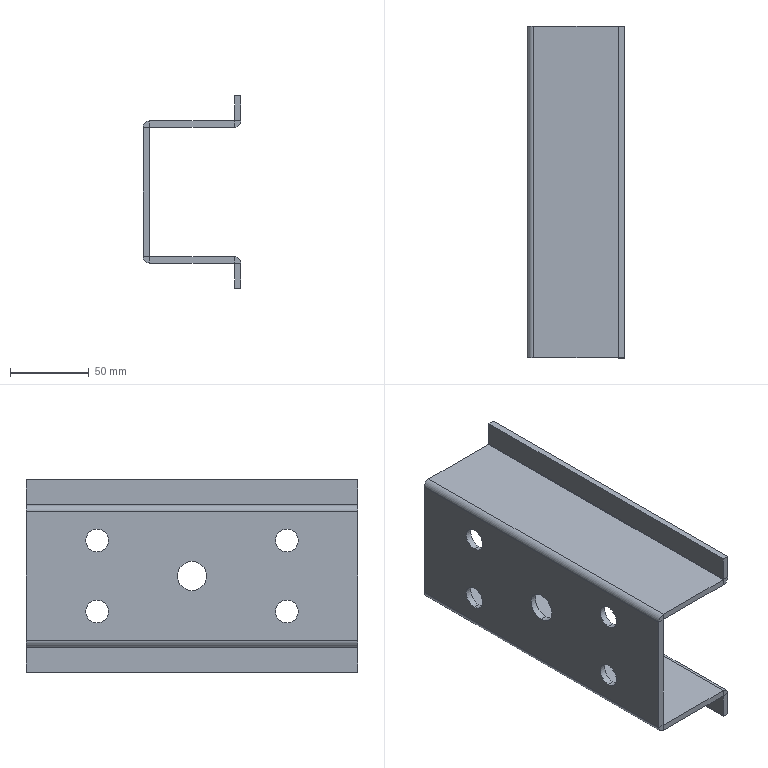Part | 1 solid | 48 faces | box 62 x 210 x 122 mm | volume 193030 mm3 | plane 30 | cylinder 18 | commonest cylinder face diameters 14.5 x8 0.4 x4 8.4 x4 18.5 x2
STEP:
#1=CARTESIAN_POINT('',(0.,0.,-9.25));
#2=VERTEX_POINT('',#1);
#3=CARTESIAN_POINT('',(0.,0.,9.25));
#4=VERTEX_POINT('',#3);
#5=CARTESIAN_POINT('',(0.,0.,0.));
#6=DIRECTION('',(-1.,0.,0.));
#7=DIRECTION('',(0.,0.,1.));
#8=AXIS2_PLACEMENT_3D('',#5,#6,#7);
#9=CIRCLE('',#8,9.25);
#10=EDGE_CURVE('',#2,#4,#9,.T.);
#11=ORIENTED_EDGE('',*,*,#10,.T.);
#12=CARTESIAN_POINT('',(4.,0.,9.25));
#13=VERTEX_POINT('',#12);
#14=CARTESIAN_POINT('',(-6.,0.,9.25));
#15=DIRECTION('',(1.,0.,0.));
#16=VECTOR('',#15,1000.);
#17=LINE('',#14,#16);
#18=EDGE_CURVE('',#4,#13,#17,.T.);
#19=ORIENTED_EDGE('',*,*,#18,.T.);
#20=CARTESIAN_POINT('',(4.,0.,-9.25));
#21=VERTEX_POINT('',#20);
#22=CARTESIAN_POINT('',(4.,0.,0.));
#23=DIRECTION('',(1.,0.,0.));
#24=DIRECTION('',(0.,0.,-1.));
#25=AXIS2_PLACEMENT_3D('',#22,#23,#24);
#26=CIRCLE('',#25,9.25);
#27=EDGE_CURVE('',#13,#21,#26,.T.);
#28=ORIENTED_EDGE('',*,*,#27,.T.);
#29=CARTESIAN_POINT('',(-6.,0.,-9.25));
#30=DIRECTION('',(1.,0.,0.));
#31=VECTOR('',#30,1000.);
#32=LINE('',#29,#31);
#33=EDGE_CURVE('',#2,#21,#32,.T.);
#34=ORIENTED_EDGE('',*,*,#33,.F.);
#35=EDGE_LOOP('',(#11,#19,#28,#34));
#36=FACE_OUTER_BOUND('',#35,.T.);
#37=CARTESIAN_POINT('',(-6.,0.,0.));
#38=DIRECTION('',(1.,0.,0.));
#39=DIRECTION('',(0.,0.,-1.));
#40=AXIS2_PLACEMENT_3D('',#37,#38,#39);
#41=CYLINDRICAL_SURFACE('',#40,9.25);
#42=ADVANCED_FACE('',(#36),#41,.F.);
#43=CARTESIAN_POINT('',(0.,-60.,-29.75));
#44=VERTEX_POINT('',#43);
#45=CARTESIAN_POINT('',(0.,-60.,-15.25));
#46=VERTEX_POINT('',#45);
#47=CARTESIAN_POINT('',(0.,-60.,-22.5));
#48=DIRECTION('',(-1.,0.,0.));
#49=DIRECTION('',(0.,0.,1.));
#50=AXIS2_PLACEMENT_3D('',#47,#48,#49);
#51=CIRCLE('',#50,7.25);
#52=EDGE_CURVE('',#44,#46,#51,.T.);
#53=ORIENTED_EDGE('',*,*,#52,.T.);
#54=CARTESIAN_POINT('',(4.,-60.,-15.25));
#55=VERTEX_POINT('',#54);
#56=CARTESIAN_POINT('',(-6.,-60.,-15.25));
#57=DIRECTION('',(1.,0.,0.));
#58=VECTOR('',#57,1000.);
#59=LINE('',#56,#58);
#60=EDGE_CURVE('',#46,#55,#59,.T.);
#61=ORIENTED_EDGE('',*,*,#60,.T.);
#62=CARTESIAN_POINT('',(4.,-60.,-29.75));
#63=VERTEX_POINT('',#62);
#64=CARTESIAN_POINT('',(4.,-60.,-22.5));
#65=DIRECTION('',(1.,0.,0.));
#66=DIRECTION('',(0.,0.,-1.));
#67=AXIS2_PLACEMENT_3D('',#64,#65,#66);
#68=CIRCLE('',#67,7.25);
#69=EDGE_CURVE('',#55,#63,#68,.T.);
#70=ORIENTED_EDGE('',*,*,#69,.T.);
#71=CARTESIAN_POINT('',(-6.,-60.,-29.75));
#72=DIRECTION('',(1.,0.,0.));
#73=VECTOR('',#72,1000.);
#74=LINE('',#71,#73);
#75=EDGE_CURVE('',#44,#63,#74,.T.);
#76=ORIENTED_EDGE('',*,*,#75,.F.);
#77=EDGE_LOOP('',(#53,#61,#70,#76));
#78=FACE_OUTER_BOUND('',#77,.T.);
#79=CARTESIAN_POINT('',(-6.,-60.,-22.5));
#80=DIRECTION('',(1.,0.,0.));
#81=DIRECTION('',(0.,0.,-1.));
#82=AXIS2_PLACEMENT_3D('',#79,#80,#81);
#83=CYLINDRICAL_SURFACE('',#82,7.25);
#84=ADVANCED_FACE('',(#78),#83,.F.);
#85=CARTESIAN_POINT('',(0.,-60.,15.25));
#86=VERTEX_POINT('',#85);
#87=CARTESIAN_POINT('',(0.,-60.,29.75));
#88=VERTEX_POINT('',#87);
#89=CARTESIAN_POINT('',(0.,-60.,22.5));
#90=DIRECTION('',(-1.,0.,0.));
#91=DIRECTION('',(0.,0.,1.));
#92=AXIS2_PLACEMENT_3D('',#89,#90,#91);
#93=CIRCLE('',#92,7.25);
#94=EDGE_CURVE('',#86,#88,#93,.T.);
#95=ORIENTED_EDGE('',*,*,#94,.T.);
#96=CARTESIAN_POINT('',(4.,-60.,29.75));
#97=VERTEX_POINT('',#96);
#98=CARTESIAN_POINT('',(-6.,-60.,29.75));
#99=DIRECTION('',(1.,0.,0.));
#100=VECTOR('',#99,1000.);
#101=LINE('',#98,#100);
#102=EDGE_CURVE('',#88,#97,#101,.T.);
#103=ORIENTED_EDGE('',*,*,#102,.T.);
#104=CARTESIAN_POINT('',(4.,-60.,15.25));
#105=VERTEX_POINT('',#104);
#106=CARTESIAN_POINT('',(4.,-60.,22.5));
#107=DIRECTION('',(1.,0.,0.));
#108=DIRECTION('',(0.,0.,-1.));
#109=AXIS2_PLACEMENT_3D('',#106,#107,#108);
#110=CIRCLE('',#109,7.25);
#111=EDGE_CURVE('',#97,#105,#110,.T.);
#112=ORIENTED_EDGE('',*,*,#111,.T.);
#113=CARTESIAN_POINT('',(-6.,-60.,15.25));
#114=DIRECTION('',(1.,0.,0.));
#115=VECTOR('',#114,1000.);
#116=LINE('',#113,#115);
#117=EDGE_CURVE('',#86,#105,#116,.T.);
#118=ORIENTED_EDGE('',*,*,#117,.F.);
#119=EDGE_LOOP('',(#95,#103,#112,#118));
#120=FACE_OUTER_BOUND('',#119,.T.);
#121=CARTESIAN_POINT('',(-6.,-60.,22.5));
#122=DIRECTION('',(1.,0.,0.));
#123=DIRECTION('',(0.,0.,-1.));
#124=AXIS2_PLACEMENT_3D('',#121,#122,#123);
#125=CYLINDRICAL_SURFACE('',#124,7.25);
#126=ADVANCED_FACE('',(#120),#125,.F.);
#127=CARTESIAN_POINT('',(0.,60.,15.25));
#128=VERTEX_POINT('',#127);
#129=CARTESIAN_POINT('',(0.,60.,29.75));
#130=VERTEX_POINT('',#129);
#131=CARTESIAN_POINT('',(0.,60.,22.5));
#132=DIRECTION('',(-1.,0.,0.));
#133=DIRECTION('',(0.,0.,1.));
#134=AXIS2_PLACEMENT_3D('',#131,#132,#133);
#135=CIRCLE('',#134,7.25);
#136=EDGE_CURVE('',#128,#130,#135,.T.);
#137=ORIENTED_EDGE('',*,*,#136,.T.);
#138=CARTESIAN_POINT('',(4.,60.,29.75));
#139=VERTEX_POINT('',#138);
#140=CARTESIAN_POINT('',(-6.,60.,29.75));
#141=DIRECTION('',(1.,0.,0.));
#142=VECTOR('',#141,1000.);
#143=LINE('',#140,#142);
#144=EDGE_CURVE('',#130,#139,#143,.T.);
#145=ORIENTED_EDGE('',*,*,#144,.T.);
#146=CARTESIAN_POINT('',(4.,60.,15.25));
#147=VERTEX_POINT('',#146);
#148=CARTESIAN_POINT('',(4.,60.,22.5));
#149=DIRECTION('',(1.,0.,0.));
#150=DIRECTION('',(0.,0.,-1.));
#151=AXIS2_PLACEMENT_3D('',#148,#149,#150);
#152=CIRCLE('',#151,7.25);
#153=EDGE_CURVE('',#139,#147,#152,.T.);
#154=ORIENTED_EDGE('',*,*,#153,.T.);
#155=CARTESIAN_POINT('',(-6.,60.,15.25));
#156=DIRECTION('',(1.,0.,0.));
#157=VECTOR('',#156,1000.);
#158=LINE('',#155,#157);
#159=EDGE_CURVE('',#128,#147,#158,.T.);
#160=ORIENTED_EDGE('',*,*,#159,.F.);
#161=EDGE_LOOP('',(#137,#145,#154,#160));
#162=FACE_OUTER_BOUND('',#161,.T.);
#163=CARTESIAN_POINT('',(-6.,60.,22.5));
#164=DIRECTION('',(1.,0.,0.));
#165=DIRECTION('',(0.,0.,-1.));
#166=AXIS2_PLACEMENT_3D('',#163,#164,#165);
#167=CYLINDRICAL_SURFACE('',#166,7.25);
#168=ADVANCED_FACE('',(#162),#167,.F.);
#169=CARTESIAN_POINT('',(0.,60.,-29.75));
#170=VERTEX_POINT('',#169);
#171=CARTESIAN_POINT('',(0.,60.,-15.25));
#172=VERTEX_POINT('',#171);
#173=CARTESIAN_POINT('',(0.,60.,-22.5));
#174=DIRECTION('',(-1.,0.,0.));
#175=DIRECTION('',(0.,0.,1.));
#176=AXIS2_PLACEMENT_3D('',#173,#174,#175);
#177=CIRCLE('',#176,7.25);
#178=EDGE_CURVE('',#170,#172,#177,.T.);
#179=ORIENTED_EDGE('',*,*,#178,.T.);
#180=CARTESIAN_POINT('',(4.,60.,-15.25));
#181=VERTEX_POINT('',#180);
#182=CARTESIAN_POINT('',(-6.,60.,-15.25));
#183=DIRECTION('',(1.,0.,0.));
#184=VECTOR('',#183,1000.);
#185=LINE('',#182,#184);
#186=EDGE_CURVE('',#172,#181,#185,.T.);
#187=ORIENTED_EDGE('',*,*,#186,.T.);
#188=CARTESIAN_POINT('',(4.,60.,-29.75));
#189=VERTEX_POINT('',#188);
#190=CARTESIAN_POINT('',(4.,60.,-22.5));
#191=DIRECTION('',(1.,0.,0.));
#192=DIRECTION('',(0.,0.,-1.));
#193=AXIS2_PLACEMENT_3D('',#190,#191,#192);
#194=CIRCLE('',#193,7.25);
#195=EDGE_CURVE('',#181,#189,#194,.T.);
#196=ORIENTED_EDGE('',*,*,#195,.T.);
#197=CARTESIAN_POINT('',(-6.,60.,-29.75));
#198=DIRECTION('',(1.,0.,0.));
#199=VECTOR('',#198,1000.);
#200=LINE('',#197,#199);
#201=EDGE_CURVE('',#170,#189,#200,.T.);
#202=ORIENTED_EDGE('',*,*,#201,.F.);
#203=EDGE_LOOP('',(#179,#187,#196,#202));
#204=FACE_OUTER_BOUND('',#203,.T.);
#205=CARTESIAN_POINT('',(-6.,60.,-22.5));
#206=DIRECTION('',(1.,0.,0.));
#207=DIRECTION('',(0.,0.,-1.));
#208=AXIS2_PLACEMENT_3D('',#205,#206,#207);
#209=CYLINDRICAL_SURFACE('',#208,7.25);
#210=ADVANCED_FACE('',(#204),#209,.F.);
#211=CARTESIAN_POINT('',(57.8,-105.,45.));
#212=VERTEX_POINT('',#211);
#213=CARTESIAN_POINT('',(4.2,-105.,45.));
#214=VERTEX_POINT('',#213);
#215=CARTESIAN_POINT('',(0.,-105.,45.));
#216=DIRECTION('',(-1.,0.,0.));
#217=VECTOR('',#216,1000.);
#218=LINE('',#215,#217);
#219=EDGE_CURVE('',#212,#214,#218,.T.);
#220=ORIENTED_EDGE('',*,*,#219,.F.);
#221=CARTESIAN_POINT('',(57.8,105.,45.));
#222=VERTEX_POINT('',#221);
#223=CARTESIAN_POINT('',(57.8,105.,45.));
#224=DIRECTION('',(0.,-1.,0.));
#225=VECTOR('',#224,1000.);
#226=LINE('',#223,#225);
#227=EDGE_CURVE('',#222,#212,#226,.T.);
#228=ORIENTED_EDGE('',*,*,#227,.F.);
#229=CARTESIAN_POINT('',(4.2,105.,45.));
#230=VERTEX_POINT('',#229);
#231=CARTESIAN_POINT('',(0.,105.,45.));
#232=DIRECTION('',(-1.,0.,0.));
#233=VECTOR('',#232,1000.);
#234=LINE('',#231,#233);
#235=EDGE_CURVE('',#222,#230,#234,.T.);
#236=ORIENTED_EDGE('',*,*,#235,.T.);
#237=CARTESIAN_POINT('',(4.2,105.,45.));
#238=DIRECTION('',(0.,-1.,0.));
#239=VECTOR('',#238,1000.);
#240=LINE('',#237,#239);
#241=EDGE_CURVE('',#230,#214,#240,.T.);
#242=ORIENTED_EDGE('',*,*,#241,.T.);
#243=EDGE_LOOP('',(#220,#228,#236,#242));
#244=FACE_OUTER_BOUND('',#243,.T.);
#245=CARTESIAN_POINT('',(0.,105.,45.));
#246=DIRECTION('',(0.,0.,1.));
#247=DIRECTION('',(1.,0.,0.));
#248=AXIS2_PLACEMENT_3D('',#245,#246,#247);
#249=PLANE('',#248);
#250=ADVANCED_FACE('',(#244),#249,.T.);
#251=CARTESIAN_POINT('',(57.8,105.,41.));
#252=VERTEX_POINT('',#251);
#253=CARTESIAN_POINT('',(57.8,-105.,41.));
#254=VERTEX_POINT('',#253);
#255=CARTESIAN_POINT('',(57.8,105.,41.));
#256=DIRECTION('',(0.,-1.,0.));
#257=VECTOR('',#256,1000.);
#258=LINE('',#255,#257);
#259=EDGE_CURVE('',#252,#254,#258,.T.);
#260=ORIENTED_EDGE('',*,*,#259,.T.);
#261=CARTESIAN_POINT('',(4.2,-105.,41.));
#262=VERTEX_POINT('',#261);
#263=CARTESIAN_POINT('',(0.,-105.,41.));
#264=DIRECTION('',(-1.,0.,0.));
#265=VECTOR('',#264,1000.);
#266=LINE('',#263,#265);
#267=EDGE_CURVE('',#254,#262,#266,.T.);
#268=ORIENTED_EDGE('',*,*,#267,.T.);
#269=CARTESIAN_POINT('',(4.2,105.,41.));
#270=VERTEX_POINT('',#269);
#271=CARTESIAN_POINT('',(4.2,105.,41.));
#272=DIRECTION('',(0.,-1.,0.));
#273=VECTOR('',#272,1000.);
#274=LINE('',#271,#273);
#275=EDGE_CURVE('',#270,#262,#274,.T.);
#276=ORIENTED_EDGE('',*,*,#275,.F.);
#277=CARTESIAN_POINT('',(0.,105.,41.));
#278=DIRECTION('',(-1.,0.,0.));
#279=VECTOR('',#278,1000.);
#280=LINE('',#277,#279);
#281=EDGE_CURVE('',#252,#270,#280,.T.);
#282=ORIENTED_EDGE('',*,*,#281,.F.);
#283=EDGE_LOOP('',(#260,#268,#276,#282));
#284=FACE_OUTER_BOUND('',#283,.T.);
#285=CARTESIAN_POINT('',(0.,105.,41.));
#286=DIRECTION('',(0.,0.,1.));
#287=DIRECTION('',(1.,0.,0.));
#288=AXIS2_PLACEMENT_3D('',#285,#286,#287);
#289=PLANE('',#288);
#290=ADVANCED_FACE('',(#284),#289,.F.);
#291=ORIENTED_EDGE('',*,*,#235,.F.);
#292=CARTESIAN_POINT('',(57.8,105.,45.));
#293=DIRECTION('',(0.,0.,-1.));
#294=VECTOR('',#293,1000.);
#295=LINE('',#292,#294);
#296=EDGE_CURVE('',#222,#252,#295,.T.);
#297=ORIENTED_EDGE('',*,*,#296,.T.);
#298=ORIENTED_EDGE('',*,*,#281,.T.);
#299=CARTESIAN_POINT('',(4.2,105.,41.));
#300=DIRECTION('',(0.,0.,1.));
#301=VECTOR('',#300,1000.);
#302=LINE('',#299,#301);
#303=EDGE_CURVE('',#270,#230,#302,.T.);
#304=ORIENTED_EDGE('',*,*,#303,.T.);
#305=EDGE_LOOP('',(#291,#297,#298,#304));
#306=FACE_OUTER_BOUND('',#305,.T.);
#307=CARTESIAN_POINT('',(4.2,105.,-40.8));
#308=DIRECTION('',(0.,1.,0.));
#309=DIRECTION('',(1.,0.,0.));
#310=AXIS2_PLACEMENT_3D('',#307,#308,#309);
#311=PLANE('',#310);
#312=ADVANCED_FACE('',(#306),#311,.T.);
#313=CARTESIAN_POINT('',(57.8,-105.,-41.));
#314=VERTEX_POINT('',#313);
#315=CARTESIAN_POINT('',(57.8,105.,-41.));
#316=VERTEX_POINT('',#315);
#317=CARTESIAN_POINT('',(57.8,-105.,-41.));
#318=DIRECTION('',(0.,1.,0.));
#319=VECTOR('',#318,1000.);
#320=LINE('',#317,#319);
#321=EDGE_CURVE('',#314,#316,#320,.T.);
#322=ORIENTED_EDGE('',*,*,#321,.T.);
#323=CARTESIAN_POINT('',(4.2,105.,-41.));
#324=VERTEX_POINT('',#323);
#325=CARTESIAN_POINT('',(0.,105.,-41.));
#326=DIRECTION('',(1.,0.,0.));
#327=VECTOR('',#326,1000.);
#328=LINE('',#325,#327);
#329=EDGE_CURVE('',#324,#316,#328,.T.);
#330=ORIENTED_EDGE('',*,*,#329,.F.);
#331=CARTESIAN_POINT('',(4.2,-105.,-41.));
#332=VERTEX_POINT('',#331);
#333=CARTESIAN_POINT('',(4.2,105.,-41.));
#334=DIRECTION('',(0.,-1.,0.));
#335=VECTOR('',#334,1000.);
#336=LINE('',#333,#335);
#337=EDGE_CURVE('',#324,#332,#336,.T.);
#338=ORIENTED_EDGE('',*,*,#337,.T.);
#339=CARTESIAN_POINT('',(0.,-105.,-41.));
#340=DIRECTION('',(1.,0.,0.));
#341=VECTOR('',#340,1000.);
#342=LINE('',#339,#341);
#343=EDGE_CURVE('',#332,#314,#342,.T.);
#344=ORIENTED_EDGE('',*,*,#343,.T.);
#345=EDGE_LOOP('',(#322,#330,#338,#344));
#346=FACE_OUTER_BOUND('',#345,.T.);
#347=CARTESIAN_POINT('',(0.,105.,-41.));
#348=DIRECTION('',(0.,0.,-1.));
#349=DIRECTION('',(-1.,0.,0.));
#350=AXIS2_PLACEMENT_3D('',#347,#348,#349);
#351=PLANE('',#350);
#352=ADVANCED_FACE('',(#346),#351,.F.);
#353=CARTESIAN_POINT('',(4.2,105.,-45.));
#354=VERTEX_POINT('',#353);
#355=CARTESIAN_POINT('',(57.8,105.,-45.));
#356=VERTEX_POINT('',#355);
#357=CARTESIAN_POINT('',(0.,105.,-45.));
#358=DIRECTION('',(1.,0.,0.));
#359=VECTOR('',#358,1000.);
#360=LINE('',#357,#359);
#361=EDGE_CURVE('',#354,#356,#360,.T.);
#362=ORIENTED_EDGE('',*,*,#361,.T.);
#363=CARTESIAN_POINT('',(57.8,-105.,-45.));
#364=VERTEX_POINT('',#363);
#365=CARTESIAN_POINT('',(57.8,-105.,-45.));
#366=DIRECTION('',(0.,1.,0.));
#367=VECTOR('',#366,1000.);
#368=LINE('',#365,#367);
#369=EDGE_CURVE('',#364,#356,#368,.T.);
#370=ORIENTED_EDGE('',*,*,#369,.F.);
#371=CARTESIAN_POINT('',(4.2,-105.,-45.));
#372=VERTEX_POINT('',#371);
#373=CARTESIAN_POINT('',(0.,-105.,-45.));
#374=DIRECTION('',(1.,0.,0.));
#375=VECTOR('',#374,1000.);
#376=LINE('',#373,#375);
#377=EDGE_CURVE('',#372,#364,#376,.T.);
#378=ORIENTED_EDGE('',*,*,#377,.F.);
#379=CARTESIAN_POINT('',(4.2,105.,-45.));
#380=DIRECTION('',(0.,-1.,0.));
#381=VECTOR('',#380,1000.);
#382=LINE('',#379,#381);
#383=EDGE_CURVE('',#354,#372,#382,.T.);
#384=ORIENTED_EDGE('',*,*,#383,.F.);
#385=EDGE_LOOP('',(#362,#370,#378,#384));
#386=FACE_OUTER_BOUND('',#385,.T.);
#387=CARTESIAN_POINT('',(0.,105.,-45.));
#388=DIRECTION('',(0.,0.,-1.));
#389=DIRECTION('',(-1.,0.,0.));
#390=AXIS2_PLACEMENT_3D('',#387,#388,#389);
#391=PLANE('',#390);
#392=ADVANCED_FACE('',(#386),#391,.T.);
#393=CARTESIAN_POINT('',(57.8,-105.,-45.));
#394=DIRECTION('',(0.,0.,1.));
#395=VECTOR('',#394,1000.);
#396=LINE('',#393,#395);
#397=EDGE_CURVE('',#364,#314,#396,.T.);
#398=ORIENTED_EDGE('',*,*,#397,.T.);
#399=ORIENTED_EDGE('',*,*,#343,.F.);
#400=CARTESIAN_POINT('',(4.2,-105.,-41.));
#401=DIRECTION('',(0.,0.,-1.));
#402=VECTOR('',#401,1000.);
#403=LINE('',#400,#402);
#404=EDGE_CURVE('',#332,#372,#403,.T.);
#405=ORIENTED_EDGE('',*,*,#404,.T.);
#406=ORIENTED_EDGE('',*,*,#377,.T.);
#407=EDGE_LOOP('',(#398,#399,#405,#406));
#408=FACE_OUTER_BOUND('',#407,.T.);
#409=CARTESIAN_POINT('',(4.2,-105.,-40.8));
#410=DIRECTION('',(0.,1.,0.));
#411=DIRECTION('',(1.,0.,0.));
#412=AXIS2_PLACEMENT_3D('',#409,#410,#411);
#413=PLANE('',#412);
#414=ADVANCED_FACE('',(#408),#413,.F.);
#415=CARTESIAN_POINT('',(0.,105.,40.8));
#416=VERTEX_POINT('',#415);
#417=CARTESIAN_POINT('',(4.,105.,40.8));
#418=VERTEX_POINT('',#417);
#419=CARTESIAN_POINT('',(0.,105.,40.8));
#420=DIRECTION('',(1.,0.,0.));
#421=VECTOR('',#420,1000.);
#422=LINE('',#419,#421);
#423=EDGE_CURVE('',#416,#418,#422,.T.);
#424=ORIENTED_EDGE('',*,*,#423,.F.);
#425=CARTESIAN_POINT('',(4.2,105.,40.8));
#426=DIRECTION('',(0.,-1.,0.));
#427=DIRECTION('',(0.,0.,1.));
#428=AXIS2_PLACEMENT_3D('',#425,#426,#427);
#429=CIRCLE('',#428,4.2);
#430=EDGE_CURVE('',#230,#416,#429,.T.);
#431=ORIENTED_EDGE('',*,*,#430,.F.);
#432=ORIENTED_EDGE('',*,*,#303,.F.);
#433=CARTESIAN_POINT('',(4.2,105.,40.8));
#434=DIRECTION('',(0.,-1.,0.));
#435=DIRECTION('',(1.,0.,0.));
#436=AXIS2_PLACEMENT_3D('',#433,#434,#435);
#437=CIRCLE('',#436,0.2);
#438=EDGE_CURVE('',#270,#418,#437,.T.);
#439=ORIENTED_EDGE('',*,*,#438,.T.);
#440=EDGE_LOOP('',(#424,#431,#432,#439));
#441=FACE_OUTER_BOUND('',#440,.T.);
#442=CARTESIAN_POINT('',(0.,105.,40.8));
#443=DIRECTION('',(0.,1.,0.));
#444=DIRECTION('',(0.,0.,1.));
#445=AXIS2_PLACEMENT_3D('',#442,#443,#444);
#446=PLANE('',#445);
#447=ADVANCED_FACE('',(#441),#446,.T.);
#448=CARTESIAN_POINT('',(0.,105.,-40.8));
#449=VERTEX_POINT('',#448);
#450=CARTESIAN_POINT('',(0.,105.,-45.));
#451=DIRECTION('',(0.,0.,-1.));
#452=VECTOR('',#451,1000.);
#453=LINE('',#450,#452);
#454=EDGE_CURVE('',#416,#449,#453,.T.);
#455=ORIENTED_EDGE('',*,*,#454,.F.);
#456=ORIENTED_EDGE('',*,*,#423,.T.);
#457=CARTESIAN_POINT('',(4.,105.,-40.8));
#458=VERTEX_POINT('',#457);
#459=CARTESIAN_POINT('',(4.,105.,-45.));
#460=DIRECTION('',(0.,0.,-1.));
#461=VECTOR('',#460,1000.);
#462=LINE('',#459,#461);
#463=EDGE_CURVE('',#418,#458,#462,.T.);
#464=ORIENTED_EDGE('',*,*,#463,.T.);
#465=CARTESIAN_POINT('',(4.,105.,-40.8));
#466=DIRECTION('',(-1.,0.,0.));
#467=VECTOR('',#466,1000.);
#468=LINE('',#465,#467);
#469=EDGE_CURVE('',#458,#449,#468,.T.);
#470=ORIENTED_EDGE('',*,*,#469,.T.);
#471=EDGE_LOOP('',(#455,#456,#464,#470));
#472=FACE_OUTER_BOUND('',#471,.T.);
#473=CARTESIAN_POINT('',(4.2,105.,41.));
#474=DIRECTION('',(0.,1.,0.));
#475=DIRECTION('',(0.,0.,1.));
#476=AXIS2_PLACEMENT_3D('',#473,#474,#475);
#477=PLANE('',#476);
#478=ADVANCED_FACE('',(#472),#477,.T.);
#479=CARTESIAN_POINT('',(4.2,-105.,45.));
#480=DIRECTION('',(0.,0.,-1.));
#481=VECTOR('',#480,1000.);
#482=LINE('',#479,#481);
#483=EDGE_CURVE('',#214,#262,#482,.T.);
#484=ORIENTED_EDGE('',*,*,#483,.F.);
#485=CARTESIAN_POINT('',(0.,-105.,40.8));
#486=VERTEX_POINT('',#485);
#487=CARTESIAN_POINT('',(4.2,-105.,40.8));
#488=DIRECTION('',(0.,-1.,0.));
#489=DIRECTION('',(0.,0.,1.));
#490=AXIS2_PLACEMENT_3D('',#487,#488,#489);
#491=CIRCLE('',#490,4.2);
#492=EDGE_CURVE('',#214,#486,#491,.T.);
#493=ORIENTED_EDGE('',*,*,#492,.T.);
#494=CARTESIAN_POINT('',(4.,-105.,40.8));
#495=VERTEX_POINT('',#494);
#496=CARTESIAN_POINT('',(4.,-105.,40.8));
#497=DIRECTION('',(-1.,0.,0.));
#498=VECTOR('',#497,1000.);
#499=LINE('',#496,#498);
#500=EDGE_CURVE('',#495,#486,#499,.T.);
#501=ORIENTED_EDGE('',*,*,#500,.F.);
#502=CARTESIAN_POINT('',(4.2,-105.,40.8));
#503=DIRECTION('',(0.,-1.,0.));
#504=DIRECTION('',(1.,0.,0.));
#505=AXIS2_PLACEMENT_3D('',#502,#503,#504);
#506=CIRCLE('',#505,0.2);
#507=EDGE_CURVE('',#262,#495,#506,.T.);
#508=ORIENTED_EDGE('',*,*,#507,.F.);
#509=EDGE_LOOP('',(#484,#493,#501,#508));
#510=FACE_OUTER_BOUND('',#509,.T.);
#511=CARTESIAN_POINT('',(4.2,-105.,45.));
#512=DIRECTION('',(0.,-1.,0.));
#513=DIRECTION('',(0.,0.,-1.));
#514=AXIS2_PLACEMENT_3D('',#511,#512,#513);
#515=PLANE('',#514);
#516=ADVANCED_FACE('',(#510),#515,.T.);
#517=CARTESIAN_POINT('',(57.8,-105.,45.));
#518=DIRECTION('',(0.,0.,-1.));
#519=VECTOR('',#518,1000.);
#520=LINE('',#517,#519);
#521=EDGE_CURVE('',#212,#254,#520,.T.);
#522=ORIENTED_EDGE('',*,*,#521,.F.);
#523=ORIENTED_EDGE('',*,*,#219,.T.);
#524=ORIENTED_EDGE('',*,*,#483,.T.);
#525=ORIENTED_EDGE('',*,*,#267,.F.);
#526=EDGE_LOOP('',(#522,#523,#524,#525));
#527=FACE_OUTER_BOUND('',#526,.T.);
#528=CARTESIAN_POINT('',(4.,-105.,40.8));
#529=DIRECTION('',(0.,-1.,0.));
#530=DIRECTION('',(0.,0.,-1.));
#531=AXIS2_PLACEMENT_3D('',#528,#529,#530);
#532=PLANE('',#531);
#533=ADVANCED_FACE('',(#527),#532,.T.);
#534=CARTESIAN_POINT('',(4.2,105.,-45.));
#535=DIRECTION('',(0.,0.,1.));
#536=VECTOR('',#535,1000.);
#537=LINE('',#534,#536);
#538=EDGE_CURVE('',#354,#324,#537,.T.);
#539=ORIENTED_EDGE('',*,*,#538,.F.);
#540=CARTESIAN_POINT('',(4.2,105.,-40.8));
#541=DIRECTION('',(0.,-1.,0.));
#542=DIRECTION('',(0.,0.,1.));
#543=AXIS2_PLACEMENT_3D('',#540,#541,#542);
#544=CIRCLE('',#543,4.2);
#545=EDGE_CURVE('',#449,#354,#544,.T.);
#546=ORIENTED_EDGE('',*,*,#545,.F.);
#547=ORIENTED_EDGE('',*,*,#469,.F.);
#548=CARTESIAN_POINT('',(4.2,105.,-40.8));
#549=DIRECTION('',(0.,-1.,0.));
#550=DIRECTION('',(1.,0.,0.));
#551=AXIS2_PLACEMENT_3D('',#548,#549,#550);
#552=CIRCLE('',#551,0.2);
#553=EDGE_CURVE('',#458,#324,#552,.T.);
#554=ORIENTED_EDGE('',*,*,#553,.T.);
#555=EDGE_LOOP('',(#539,#546,#547,#554));
#556=FACE_OUTER_BOUND('',#555,.T.);
#557=CARTESIAN_POINT('',(4.2,105.,-45.));
#558=DIRECTION('',(0.,1.,0.));
#559=DIRECTION('',(0.,0.,1.));
#560=AXIS2_PLACEMENT_3D('',#557,#558,#559);
#561=PLANE('',#560);
#562=ADVANCED_FACE('',(#556),#561,.T.);
#563=CARTESIAN_POINT('',(57.8,105.,-45.));
#564=DIRECTION('',(0.,0.,1.));
#565=VECTOR('',#564,1000.);
#566=LINE('',#563,#565);
#567=EDGE_CURVE('',#356,#316,#566,.T.);
#568=ORIENTED_EDGE('',*,*,#567,.F.);
#569=ORIENTED_EDGE('',*,*,#361,.F.);
#570=ORIENTED_EDGE('',*,*,#538,.T.);
#571=ORIENTED_EDGE('',*,*,#329,.T.);
#572=EDGE_LOOP('',(#568,#569,#570,#571));
#573=FACE_OUTER_BOUND('',#572,.T.);
#574=CARTESIAN_POINT('',(4.,105.,-40.8));
#575=DIRECTION('',(0.,1.,0.));
#576=DIRECTION('',(0.,0.,1.));
#577=AXIS2_PLACEMENT_3D('',#574,#575,#576);
#578=PLANE('',#577);
#579=ADVANCED_FACE('',(#573),#578,.T.);
#580=CARTESIAN_POINT('',(0.,-105.,-40.8));
#581=VERTEX_POINT('',#580);
#582=CARTESIAN_POINT('',(4.,-105.,-40.8));
#583=VERTEX_POINT('',#582);
#584=CARTESIAN_POINT('',(0.,-105.,-40.8));
#585=DIRECTION('',(1.,0.,0.));
#586=VECTOR('',#585,1000.);
#587=LINE('',#584,#586);
#588=EDGE_CURVE('',#581,#583,#587,.T.);
#589=ORIENTED_EDGE('',*,*,#588,.F.);
#590=CARTESIAN_POINT('',(4.2,-105.,-40.8));
#591=DIRECTION('',(0.,-1.,0.));
#592=DIRECTION('',(0.,0.,1.));
#593=AXIS2_PLACEMENT_3D('',#590,#591,#592);
#594=CIRCLE('',#593,4.2);
#595=EDGE_CURVE('',#581,#372,#594,.T.);
#596=ORIENTED_EDGE('',*,*,#595,.T.);
#597=ORIENTED_EDGE('',*,*,#404,.F.);
#598=CARTESIAN_POINT('',(4.2,-105.,-40.8));
#599=DIRECTION('',(0.,-1.,0.));
#600=DIRECTION('',(1.,0.,0.));
#601=AXIS2_PLACEMENT_3D('',#598,#599,#600);
#602=CIRCLE('',#601,0.2);
#603=EDGE_CURVE('',#583,#332,#602,.T.);
#604=ORIENTED_EDGE('',*,*,#603,.F.);
#605=EDGE_LOOP('',(#589,#596,#597,#604));
#606=FACE_OUTER_BOUND('',#605,.T.);
#607=CARTESIAN_POINT('',(0.,-105.,-40.8));
#608=DIRECTION('',(0.,-1.,0.));
#609=DIRECTION('',(0.,0.,-1.));
#610=AXIS2_PLACEMENT_3D('',#607,#608,#609);
#611=PLANE('',#610);
#612=ADVANCED_FACE('',(#606),#611,.T.);
#613=CARTESIAN_POINT('',(0.,-105.,-45.));
#614=DIRECTION('',(0.,0.,-1.));
#615=VECTOR('',#614,1000.);
#616=LINE('',#613,#615);
#617=EDGE_CURVE('',#486,#581,#616,.T.);
#618=ORIENTED_EDGE('',*,*,#617,.T.);
#619=ORIENTED_EDGE('',*,*,#588,.T.);
#620=CARTESIAN_POINT('',(4.,-105.,-45.));
#621=DIRECTION('',(0.,0.,-1.));
#622=VECTOR('',#621,1000.);
#623=LINE('',#620,#622);
#624=EDGE_CURVE('',#495,#583,#623,.T.);
#625=ORIENTED_EDGE('',*,*,#624,.F.);
#626=ORIENTED_EDGE('',*,*,#500,.T.);
#627=EDGE_LOOP('',(#618,#619,#625,#626));
#628=FACE_OUTER_BOUND('',#627,.T.);
#629=CARTESIAN_POINT('',(4.2,-105.,-41.));
#630=DIRECTION('',(0.,-1.,0.));
#631=DIRECTION('',(0.,0.,-1.));
#632=AXIS2_PLACEMENT_3D('',#629,#630,#631);
#633=PLANE('',#632);
#634=ADVANCED_FACE('',(#628),#633,.T.);
#635=ORIENTED_EDGE('',*,*,#595,.F.);
#636=CARTESIAN_POINT('',(0.,105.,-40.8));
#637=DIRECTION('',(0.,-1.,0.));
#638=VECTOR('',#637,1000.);
#639=LINE('',#636,#638);
#640=EDGE_CURVE('',#449,#581,#639,.T.);
#641=ORIENTED_EDGE('',*,*,#640,.F.);
#642=ORIENTED_EDGE('',*,*,#545,.T.);
#643=ORIENTED_EDGE('',*,*,#383,.T.);
#644=EDGE_LOOP('',(#635,#641,#642,#643));
#645=FACE_OUTER_BOUND('',#644,.T.);
#646=CARTESIAN_POINT('',(4.2,105.,-40.8));
#647=DIRECTION('',(0.,-1.,0.));
#648=DIRECTION('',(0.,0.,-1.));
#649=AXIS2_PLACEMENT_3D('',#646,#647,#648);
#650=CYLINDRICAL_SURFACE('',#649,4.2);
#651=ADVANCED_FACE('',(#645),#650,.T.);
#652=ORIENTED_EDGE('',*,*,#10,.F.);
#653=CARTESIAN_POINT('',(0.,0.,0.));
#654=DIRECTION('',(-1.,0.,0.));
#655=DIRECTION('',(0.,0.,1.));
#656=AXIS2_PLACEMENT_3D('',#653,#654,#655);
#657=CIRCLE('',#656,9.25);
#658=EDGE_CURVE('',#4,#2,#657,.T.);
#659=ORIENTED_EDGE('',*,*,#658,.F.);
#660=EDGE_LOOP('',(#652,#659));
#661=FACE_BOUND('',#660,.T.);
#662=ORIENTED_EDGE('',*,*,#52,.F.);
#663=CARTESIAN_POINT('',(0.,-60.,-22.5));
#664=DIRECTION('',(-1.,0.,0.));
#665=DIRECTION('',(0.,0.,1.));
#666=AXIS2_PLACEMENT_3D('',#663,#664,#665);
#667=CIRCLE('',#666,7.25);
#668=EDGE_CURVE('',#46,#44,#667,.T.);
#669=ORIENTED_EDGE('',*,*,#668,.F.);
#670=EDGE_LOOP('',(#662,#669));
#671=FACE_BOUND('',#670,.T.);
#672=ORIENTED_EDGE('',*,*,#94,.F.);
#673=CARTESIAN_POINT('',(0.,-60.,22.5));
#674=DIRECTION('',(-1.,0.,0.));
#675=DIRECTION('',(0.,0.,1.));
#676=AXIS2_PLACEMENT_3D('',#673,#674,#675);
#677=CIRCLE('',#676,7.25);
#678=EDGE_CURVE('',#88,#86,#677,.T.);
#679=ORIENTED_EDGE('',*,*,#678,.F.);
#680=EDGE_LOOP('',(#672,#679));
#681=FACE_BOUND('',#680,.T.);
#682=ORIENTED_EDGE('',*,*,#136,.F.);
#683=CARTESIAN_POINT('',(0.,60.,22.5));
#684=DIRECTION('',(-1.,0.,0.));
#685=DIRECTION('',(0.,0.,1.));
#686=AXIS2_PLACEMENT_3D('',#683,#684,#685);
#687=CIRCLE('',#686,7.25);
#688=EDGE_CURVE('',#130,#128,#687,.T.);
#689=ORIENTED_EDGE('',*,*,#688,.F.);
#690=EDGE_LOOP('',(#682,#689));
#691=FACE_BOUND('',#690,.T.);
#692=ORIENTED_EDGE('',*,*,#178,.F.);
#693=CARTESIAN_POINT('',(0.,60.,-22.5));
#694=DIRECTION('',(-1.,0.,0.));
#695=DIRECTION('',(0.,0.,1.));
#696=AXIS2_PLACEMENT_3D('',#693,#694,#695);
#697=CIRCLE('',#696,7.25);
#698=EDGE_CURVE('',#172,#170,#697,.T.);
#699=ORIENTED_EDGE('',*,*,#698,.F.);
#700=EDGE_LOOP('',(#692,#699));
#701=FACE_BOUND('',#700,.T.);
#702=ORIENTED_EDGE('',*,*,#617,.F.);
#703=CARTESIAN_POINT('',(0.,105.,40.8));
#704=DIRECTION('',(0.,-1.,0.));
#705=VECTOR('',#704,1000.);
#706=LINE('',#703,#705);
#707=EDGE_CURVE('',#416,#486,#706,.T.);
#708=ORIENTED_EDGE('',*,*,#707,.F.);
#709=ORIENTED_EDGE('',*,*,#454,.T.);
#710=ORIENTED_EDGE('',*,*,#640,.T.);
#711=EDGE_LOOP('',(#702,#708,#709,#710));
#712=FACE_OUTER_BOUND('',#711,.T.);
#713=CARTESIAN_POINT('',(0.,105.,-45.));
#714=DIRECTION('',(-1.,0.,0.));
#715=DIRECTION('',(0.,0.,1.));
#716=AXIS2_PLACEMENT_3D('',#713,#714,#715);
#717=PLANE('',#716);
#718=ADVANCED_FACE('',(#661,#671,#681,#691,#701,#712),#717,.T.);
#719=ORIENTED_EDGE('',*,*,#492,.F.);
#720=ORIENTED_EDGE('',*,*,#241,.F.);
#721=ORIENTED_EDGE('',*,*,#430,.T.);
#722=ORIENTED_EDGE('',*,*,#707,.T.);
#723=EDGE_LOOP('',(#719,#720,#721,#722));
#724=FACE_OUTER_BOUND('',#723,.T.);
#725=CARTESIAN_POINT('',(4.2,105.,40.8));
#726=DIRECTION('',(0.,-1.,0.));
#727=DIRECTION('',(0.,0.,-1.));
#728=AXIS2_PLACEMENT_3D('',#725,#726,#727);
#729=CYLINDRICAL_SURFACE('',#728,4.2);
#730=ADVANCED_FACE('',(#724),#729,.T.);
#731=ORIENTED_EDGE('',*,*,#507,.T.);
#732=CARTESIAN_POINT('',(4.,105.,40.8));
#733=DIRECTION('',(0.,-1.,0.));
#734=VECTOR('',#733,1000.);
#735=LINE('',#732,#734);
#736=EDGE_CURVE('',#418,#495,#735,.T.);
#737=ORIENTED_EDGE('',*,*,#736,.F.);
#738=ORIENTED_EDGE('',*,*,#438,.F.);
#739=ORIENTED_EDGE('',*,*,#275,.T.);
#740=EDGE_LOOP('',(#731,#737,#738,#739));
#741=FACE_OUTER_BOUND('',#740,.T.);
#742=CARTESIAN_POINT('',(4.2,105.,40.8));
#743=DIRECTION('',(0.,-1.,0.));
#744=DIRECTION('',(0.,0.,-1.));
#745=AXIS2_PLACEMENT_3D('',#742,#743,#744);
#746=CYLINDRICAL_SURFACE('',#745,0.2);
#747=ADVANCED_FACE('',(#741),#746,.F.);
#748=CARTESIAN_POINT('',(4.,0.,0.));
#749=DIRECTION('',(1.,0.,0.));
#750=DIRECTION('',(0.,0.,-1.));
#751=AXIS2_PLACEMENT_3D('',#748,#749,#750);
#752=CIRCLE('',#751,9.25);
#753=EDGE_CURVE('',#21,#13,#752,.T.);
#754=ORIENTED_EDGE('',*,*,#753,.F.);
#755=ORIENTED_EDGE('',*,*,#27,.F.);
#756=EDGE_LOOP('',(#754,#755));
#757=FACE_BOUND('',#756,.T.);
#758=CARTESIAN_POINT('',(4.,-60.,-22.5));
#759=DIRECTION('',(1.,0.,0.));
#760=DIRECTION('',(0.,0.,-1.));
#761=AXIS2_PLACEMENT_3D('',#758,#759,#760);
#762=CIRCLE('',#761,7.25);
#763=EDGE_CURVE('',#63,#55,#762,.T.);
#764=ORIENTED_EDGE('',*,*,#763,.F.);
#765=ORIENTED_EDGE('',*,*,#69,.F.);
#766=EDGE_LOOP('',(#764,#765));
#767=FACE_BOUND('',#766,.T.);
#768=CARTESIAN_POINT('',(4.,-60.,22.5));
#769=DIRECTION('',(1.,0.,0.));
#770=DIRECTION('',(0.,0.,-1.));
#771=AXIS2_PLACEMENT_3D('',#768,#769,#770);
#772=CIRCLE('',#771,7.25);
#773=EDGE_CURVE('',#105,#97,#772,.T.);
#774=ORIENTED_EDGE('',*,*,#773,.F.);
#775=ORIENTED_EDGE('',*,*,#111,.F.);
#776=EDGE_LOOP('',(#774,#775));
#777=FACE_BOUND('',#776,.T.);
#778=CARTESIAN_POINT('',(4.,60.,22.5));
#779=DIRECTION('',(1.,0.,0.));
#780=DIRECTION('',(0.,0.,-1.));
#781=AXIS2_PLACEMENT_3D('',#778,#779,#780);
#782=CIRCLE('',#781,7.25);
#783=EDGE_CURVE('',#147,#139,#782,.T.);
#784=ORIENTED_EDGE('',*,*,#783,.F.);
#785=ORIENTED_EDGE('',*,*,#153,.F.);
#786=EDGE_LOOP('',(#784,#785));
#787=FACE_BOUND('',#786,.T.);
#788=CARTESIAN_POINT('',(4.,60.,-22.5));
#789=DIRECTION('',(1.,0.,0.));
#790=DIRECTION('',(0.,0.,-1.));
#791=AXIS2_PLACEMENT_3D('',#788,#789,#790);
#792=CIRCLE('',#791,7.25);
#793=EDGE_CURVE('',#189,#181,#792,.T.);
#794=ORIENTED_EDGE('',*,*,#793,.F.);
#795=ORIENTED_EDGE('',*,*,#195,.F.);
#796=EDGE_LOOP('',(#794,#795));
#797=FACE_BOUND('',#796,.T.);
#798=ORIENTED_EDGE('',*,*,#624,.T.);
#799=CARTESIAN_POINT('',(4.,105.,-40.8));
#800=DIRECTION('',(0.,-1.,0.));
#801=VECTOR('',#800,1000.);
#802=LINE('',#799,#801);
#803=EDGE_CURVE('',#458,#583,#802,.T.);
#804=ORIENTED_EDGE('',*,*,#803,.F.);
#805=ORIENTED_EDGE('',*,*,#463,.F.);
#806=ORIENTED_EDGE('',*,*,#736,.T.);
#807=EDGE_LOOP('',(#798,#804,#805,#806));
#808=FACE_OUTER_BOUND('',#807,.T.);
#809=CARTESIAN_POINT('',(4.,105.,-45.));
#810=DIRECTION('',(-1.,0.,0.));
#811=DIRECTION('',(0.,0.,1.));
#812=AXIS2_PLACEMENT_3D('',#809,#810,#811);
#813=PLANE('',#812);
#814=ADVANCED_FACE('',(#757,#767,#777,#787,#797,#808),#813,.F.);
#815=ORIENTED_EDGE('',*,*,#603,.T.);
#816=ORIENTED_EDGE('',*,*,#337,.F.);
#817=ORIENTED_EDGE('',*,*,#553,.F.);
#818=ORIENTED_EDGE('',*,*,#803,.T.);
#819=EDGE_LOOP('',(#815,#816,#817,#818));
#820=FACE_OUTER_BOUND('',#819,.T.);
#821=CARTESIAN_POINT('',(4.2,105.,-40.8));
#822=DIRECTION('',(0.,-1.,0.));
#823=DIRECTION('',(0.,0.,-1.));
#824=AXIS2_PLACEMENT_3D('',#821,#822,#823);
#825=CYLINDRICAL_SURFACE('',#824,0.2);
#826=ADVANCED_FACE('',(#820),#825,.F.);
#827=CARTESIAN_POINT('',(58.,105.,-45.2));
#828=VERTEX_POINT('',#827);
#829=CARTESIAN_POINT('',(62.,105.,-45.2));
#830=VERTEX_POINT('',#829);
#831=CARTESIAN_POINT('',(62.,105.,-45.2));
#832=DIRECTION('',(1.,0.,0.));
#833=VECTOR('',#832,1000.);
#834=LINE('',#831,#833);
#835=EDGE_CURVE('',#828,#830,#834,.T.);
#836=ORIENTED_EDGE('',*,*,#835,.F.);
#837=CARTESIAN_POINT('',(57.8,105.,-45.2));
#838=DIRECTION('',(0.,1.,0.));
#839=DIRECTION('',(0.,0.,-1.));
#840=AXIS2_PLACEMENT_3D('',#837,#838,#839);
#841=CIRCLE('',#840,0.2);
#842=EDGE_CURVE('',#356,#828,#841,.T.);
#843=ORIENTED_EDGE('',*,*,#842,.F.);
#844=ORIENTED_EDGE('',*,*,#567,.T.);
#845=CARTESIAN_POINT('',(57.8,105.,-45.2));
#846=DIRECTION('',(0.,1.,0.));
#847=DIRECTION('',(0.,0.,-1.));
#848=AXIS2_PLACEMENT_3D('',#845,#846,#847);
#849=CIRCLE('',#848,4.2);
#850=EDGE_CURVE('',#316,#830,#849,.T.);
#851=ORIENTED_EDGE('',*,*,#850,.T.);
#852=EDGE_LOOP('',(#836,#843,#844,#851));
#853=FACE_OUTER_BOUND('',#852,.T.);
#854=CARTESIAN_POINT('',(57.8,105.,-45.2));
#855=DIRECTION('',(0.,1.,0.));
#856=DIRECTION('',(0.,0.,1.));
#857=AXIS2_PLACEMENT_3D('',#854,#855,#856);
#858=PLANE('',#857);
#859=ADVANCED_FACE('',(#853),#858,.T.);
#860=CARTESIAN_POINT('',(58.,-105.,-45.2));
#861=VERTEX_POINT('',#860);
#862=CARTESIAN_POINT('',(57.8,-105.,-45.2));
#863=DIRECTION('',(0.,-1.,0.));
#864=DIRECTION('',(0.,0.,-1.));
#865=AXIS2_PLACEMENT_3D('',#862,#863,#864);
#866=CIRCLE('',#865,0.2);
#867=EDGE_CURVE('',#861,#364,#866,.T.);
#868=ORIENTED_EDGE('',*,*,#867,.F.);
#869=CARTESIAN_POINT('',(62.,-105.,-45.2));
#870=VERTEX_POINT('',#869);
#871=CARTESIAN_POINT('',(58.,-105.,-45.2));
#872=DIRECTION('',(1.,0.,0.));
#873=VECTOR('',#872,1000.);
#874=LINE('',#871,#873);
#875=EDGE_CURVE('',#861,#870,#874,.T.);
#876=ORIENTED_EDGE('',*,*,#875,.T.);
#877=CARTESIAN_POINT('',(57.8,-105.,-45.2));
#878=DIRECTION('',(0.,-1.,0.));
#879=DIRECTION('',(0.,0.,-1.));
#880=AXIS2_PLACEMENT_3D('',#877,#878,#879);
#881=CIRCLE('',#880,4.2);
#882=EDGE_CURVE('',#870,#314,#881,.T.);
#883=ORIENTED_EDGE('',*,*,#882,.T.);
#884=ORIENTED_EDGE('',*,*,#397,.F.);
#885=EDGE_LOOP('',(#868,#876,#883,#884));
#886=FACE_OUTER_BOUND('',#885,.T.);
#887=CARTESIAN_POINT('',(57.8,-105.,-45.2));
#888=DIRECTION('',(0.,1.,0.));
#889=DIRECTION('',(0.,0.,1.));
#890=AXIS2_PLACEMENT_3D('',#887,#888,#889);
#891=PLANE('',#890);
#892=ADVANCED_FACE('',(#886),#891,.F.);
#893=ORIENTED_EDGE('',*,*,#321,.F.);
#894=ORIENTED_EDGE('',*,*,#882,.F.);
#895=CARTESIAN_POINT('',(62.,105.,-45.2));
#896=DIRECTION('',(0.,1.,0.));
#897=VECTOR('',#896,1000.);
#898=LINE('',#895,#897);
#899=EDGE_CURVE('',#870,#830,#898,.T.);
#900=ORIENTED_EDGE('',*,*,#899,.T.);
#901=ORIENTED_EDGE('',*,*,#850,.F.);
#902=EDGE_LOOP('',(#893,#894,#900,#901));
#903=FACE_OUTER_BOUND('',#902,.T.);
#904=CARTESIAN_POINT('',(57.8,-105.,-45.2));
#905=DIRECTION('',(0.,-1.,0.));
#906=DIRECTION('',(1.,0.,0.));
#907=AXIS2_PLACEMENT_3D('',#904,#905,#906);
#908=CYLINDRICAL_SURFACE('',#907,4.2);
#909=ADVANCED_FACE('',(#903),#908,.T.);
#910=ORIENTED_EDGE('',*,*,#369,.T.);
#911=ORIENTED_EDGE('',*,*,#842,.T.);
#912=CARTESIAN_POINT('',(58.,105.,-45.2));
#913=DIRECTION('',(0.,-1.,0.));
#914=VECTOR('',#913,1000.);
#915=LINE('',#912,#914);
#916=EDGE_CURVE('',#828,#861,#915,.T.);
#917=ORIENTED_EDGE('',*,*,#916,.T.);
#918=ORIENTED_EDGE('',*,*,#867,.T.);
#919=EDGE_LOOP('',(#910,#911,#917,#918));
#920=FACE_OUTER_BOUND('',#919,.T.);
#921=CARTESIAN_POINT('',(57.8,-105.,-45.2));
#922=DIRECTION('',(0.,-1.,0.));
#923=DIRECTION('',(1.,0.,0.));
#924=AXIS2_PLACEMENT_3D('',#921,#922,#923);
#925=CYLINDRICAL_SURFACE('',#924,0.2);
#926=ADVANCED_FACE('',(#920),#925,.F.);
#927=ORIENTED_EDGE('',*,*,#875,.F.);
#928=CARTESIAN_POINT('',(58.,-105.,-61.));
#929=VERTEX_POINT('',#928);
#930=CARTESIAN_POINT('',(58.,-105.,-61.));
#931=DIRECTION('',(0.,0.,-1.));
#932=VECTOR('',#931,1000.);
#933=LINE('',#930,#932);
#934=EDGE_CURVE('',#861,#929,#933,.T.);
#935=ORIENTED_EDGE('',*,*,#934,.T.);
#936=CARTESIAN_POINT('',(62.,-105.,-61.));
#937=VERTEX_POINT('',#936);
#938=CARTESIAN_POINT('',(62.,-105.,-61.));
#939=DIRECTION('',(-1.,0.,0.));
#940=VECTOR('',#939,1000.);
#941=LINE('',#938,#940);
#942=EDGE_CURVE('',#937,#929,#941,.T.);
#943=ORIENTED_EDGE('',*,*,#942,.F.);
#944=CARTESIAN_POINT('',(62.,-105.,0.));
#945=DIRECTION('',(0.,0.,-1.));
#946=VECTOR('',#945,1000.);
#947=LINE('',#944,#946);
#948=EDGE_CURVE('',#870,#937,#947,.T.);
#949=ORIENTED_EDGE('',*,*,#948,.F.);
#950=EDGE_LOOP('',(#927,#935,#943,#949));
#951=FACE_OUTER_BOUND('',#950,.T.);
#952=CARTESIAN_POINT('',(62.,-105.,-61.));
#953=DIRECTION('',(0.,1.,0.));
#954=DIRECTION('',(0.,0.,1.));
#955=AXIS2_PLACEMENT_3D('',#952,#953,#954);
#956=PLANE('',#955);
#957=ADVANCED_FACE('',(#951),#956,.F.);
#958=ORIENTED_EDGE('',*,*,#835,.T.);
#959=CARTESIAN_POINT('',(62.,105.,-61.));
#960=VERTEX_POINT('',#959);
#961=CARTESIAN_POINT('',(62.,105.,0.));
#962=DIRECTION('',(0.,0.,1.));
#963=VECTOR('',#962,1000.);
#964=LINE('',#961,#963);
#965=EDGE_CURVE('',#960,#830,#964,.T.);
#966=ORIENTED_EDGE('',*,*,#965,.F.);
#967=CARTESIAN_POINT('',(58.,105.,-61.));
#968=VERTEX_POINT('',#967);
#969=CARTESIAN_POINT('',(62.,105.,-61.));
#970=DIRECTION('',(-1.,0.,0.));
#971=VECTOR('',#970,1000.);
#972=LINE('',#969,#971);
#973=EDGE_CURVE('',#960,#968,#972,.T.);
#974=ORIENTED_EDGE('',*,*,#973,.T.);
#975=CARTESIAN_POINT('',(58.,105.,-45.));
#976=DIRECTION('',(0.,0.,1.));
#977=VECTOR('',#976,1000.);
#978=LINE('',#975,#977);
#979=EDGE_CURVE('',#968,#828,#978,.T.);
#980=ORIENTED_EDGE('',*,*,#979,.T.);
#981=EDGE_LOOP('',(#958,#966,#974,#980));
#982=FACE_OUTER_BOUND('',#981,.T.);
#983=CARTESIAN_POINT('',(62.,105.,-45.));
#984=DIRECTION('',(0.,-1.,0.));
#985=DIRECTION('',(0.,0.,-1.));
#986=AXIS2_PLACEMENT_3D('',#983,#984,#985);
#987=PLANE('',#986);
#988=ADVANCED_FACE('',(#982),#987,.F.);
#989=ORIENTED_EDGE('',*,*,#899,.F.);
#990=ORIENTED_EDGE('',*,*,#948,.T.);
#991=CARTESIAN_POINT('',(62.,0.,-61.));
#992=DIRECTION('',(0.,1.,0.));
#993=VECTOR('',#992,1000.);
#994=LINE('',#991,#993);
#995=EDGE_CURVE('',#937,#960,#994,.T.);
#996=ORIENTED_EDGE('',*,*,#995,.T.);
#997=ORIENTED_EDGE('',*,*,#965,.T.);
#998=EDGE_LOOP('',(#989,#990,#996,#997));
#999=FACE_OUTER_BOUND('',#998,.T.);
#1000=CARTESIAN_POINT('',(62.,0.,0.));
#1001=DIRECTION('',(-1.,0.,0.));
#1002=DIRECTION('',(0.,0.,1.));
#1003=AXIS2_PLACEMENT_3D('',#1000,#1001,#1002);
#1004=PLANE('',#1003);
#1005=ADVANCED_FACE('',(#999),#1004,.F.);
#1006=ORIENTED_EDGE('',*,*,#934,.F.);
#1007=ORIENTED_EDGE('',*,*,#916,.F.);
#1008=ORIENTED_EDGE('',*,*,#979,.F.);
#1009=CARTESIAN_POINT('',(58.,105.,-61.));
#1010=DIRECTION('',(0.,1.,0.));
#1011=VECTOR('',#1010,1000.);
#1012=LINE('',#1009,#1011);
#1013=EDGE_CURVE('',#929,#968,#1012,.T.);
#1014=ORIENTED_EDGE('',*,*,#1013,.F.);
#1015=EDGE_LOOP('',(#1006,#1007,#1008,#1014));
#1016=FACE_OUTER_BOUND('',#1015,.T.);
#1017=CARTESIAN_POINT('',(58.,0.,0.));
#1018=DIRECTION('',(-1.,0.,0.));
#1019=DIRECTION('',(0.,0.,1.));
#1020=AXIS2_PLACEMENT_3D('',#1017,#1018,#1019);
#1021=PLANE('',#1020);
#1022=ADVANCED_FACE('',(#1016),#1021,.T.);
#1023=ORIENTED_EDGE('',*,*,#1013,.T.);
#1024=ORIENTED_EDGE('',*,*,#973,.F.);
#1025=ORIENTED_EDGE('',*,*,#995,.F.);
#1026=ORIENTED_EDGE('',*,*,#942,.T.);
#1027=EDGE_LOOP('',(#1023,#1024,#1025,#1026));
#1028=FACE_OUTER_BOUND('',#1027,.T.);
#1029=CARTESIAN_POINT('',(62.,105.,-61.));
#1030=DIRECTION('',(0.,0.,1.));
#1031=DIRECTION('',(1.,0.,0.));
#1032=AXIS2_PLACEMENT_3D('',#1029,#1030,#1031);
#1033=PLANE('',#1032);
#1034=ADVANCED_FACE('',(#1028),#1033,.F.);
#1035=CARTESIAN_POINT('',(58.,-105.,45.2));
#1036=VERTEX_POINT('',#1035);
#1037=CARTESIAN_POINT('',(62.,-105.,45.2));
#1038=VERTEX_POINT('',#1037);
#1039=CARTESIAN_POINT('',(62.,-105.,45.2));
#1040=DIRECTION('',(1.,0.,0.));
#1041=VECTOR('',#1040,1000.);
#1042=LINE('',#1039,#1041);
#1043=EDGE_CURVE('',#1036,#1038,#1042,.T.);
#1044=ORIENTED_EDGE('',*,*,#1043,.F.);
#1045=CARTESIAN_POINT('',(57.8,-105.,45.2));
#1046=DIRECTION('',(0.,-1.,0.));
#1047=DIRECTION('',(0.,0.,1.));
#1048=AXIS2_PLACEMENT_3D('',#1045,#1046,#1047);
#1049=CIRCLE('',#1048,0.2);
#1050=EDGE_CURVE('',#212,#1036,#1049,.T.);
#1051=ORIENTED_EDGE('',*,*,#1050,.F.);
#1052=ORIENTED_EDGE('',*,*,#521,.T.);
#1053=CARTESIAN_POINT('',(57.8,-105.,45.2));
#1054=DIRECTION('',(0.,-1.,0.));
#1055=DIRECTION('',(0.,0.,1.));
#1056=AXIS2_PLACEMENT_3D('',#1053,#1054,#1055);
#1057=CIRCLE('',#1056,4.2);
#1058=EDGE_CURVE('',#254,#1038,#1057,.T.);
#1059=ORIENTED_EDGE('',*,*,#1058,.T.);
#1060=EDGE_LOOP('',(#1044,#1051,#1052,#1059));
#1061=FACE_OUTER_BOUND('',#1060,.T.);
#1062=CARTESIAN_POINT('',(57.8,-105.,45.2));
#1063=DIRECTION('',(0.,-1.,0.));
#1064=DIRECTION('',(0.,0.,-1.));
#1065=AXIS2_PLACEMENT_3D('',#1062,#1063,#1064);
#1066=PLANE('',#1065);
#1067=ADVANCED_FACE('',(#1061),#1066,.T.);
#1068=CARTESIAN_POINT('',(58.,105.,45.2));
#1069=VERTEX_POINT('',#1068);
#1070=CARTESIAN_POINT('',(57.8,105.,45.2));
#1071=DIRECTION('',(0.,1.,0.));
#1072=DIRECTION('',(0.,0.,1.));
#1073=AXIS2_PLACEMENT_3D('',#1070,#1071,#1072);
#1074=CIRCLE('',#1073,0.2);
#1075=EDGE_CURVE('',#1069,#222,#1074,.T.);
#1076=ORIENTED_EDGE('',*,*,#1075,.F.);
#1077=CARTESIAN_POINT('',(62.,105.,45.2));
#1078=VERTEX_POINT('',#1077);
#1079=CARTESIAN_POINT('',(58.,105.,45.2));
#1080=DIRECTION('',(1.,0.,0.));
#1081=VECTOR('',#1080,1000.);
#1082=LINE('',#1079,#1081);
#1083=EDGE_CURVE('',#1069,#1078,#1082,.T.);
#1084=ORIENTED_EDGE('',*,*,#1083,.T.);
#1085=CARTESIAN_POINT('',(57.8,105.,45.2));
#1086=DIRECTION('',(0.,1.,0.));
#1087=DIRECTION('',(0.,0.,1.));
#1088=AXIS2_PLACEMENT_3D('',#1085,#1086,#1087);
#1089=CIRCLE('',#1088,4.2);
#1090=EDGE_CURVE('',#1078,#252,#1089,.T.);
#1091=ORIENTED_EDGE('',*,*,#1090,.T.);
#1092=ORIENTED_EDGE('',*,*,#296,.F.);
#1093=EDGE_LOOP('',(#1076,#1084,#1091,#1092));
#1094=FACE_OUTER_BOUND('',#1093,.T.);
#1095=CARTESIAN_POINT('',(57.8,105.,45.2));
#1096=DIRECTION('',(0.,-1.,0.));
#1097=DIRECTION('',(0.,0.,-1.));
#1098=AXIS2_PLACEMENT_3D('',#1095,#1096,#1097);
#1099=PLANE('',#1098);
#1100=ADVANCED_FACE('',(#1094),#1099,.F.);
#1101=ORIENTED_EDGE('',*,*,#259,.F.);
#1102=ORIENTED_EDGE('',*,*,#1090,.F.);
#1103=CARTESIAN_POINT('',(62.,-105.,45.2));
#1104=DIRECTION('',(0.,-1.,0.));
#1105=VECTOR('',#1104,1000.);
#1106=LINE('',#1103,#1105);
#1107=EDGE_CURVE('',#1078,#1038,#1106,.T.);
#1108=ORIENTED_EDGE('',*,*,#1107,.T.);
#1109=ORIENTED_EDGE('',*,*,#1058,.F.);
#1110=EDGE_LOOP('',(#1101,#1102,#1108,#1109));
#1111=FACE_OUTER_BOUND('',#1110,.T.);
#1112=CARTESIAN_POINT('',(57.8,105.,45.2));
#1113=DIRECTION('',(0.,1.,0.));
#1114=DIRECTION('',(1.,0.,0.));
#1115=AXIS2_PLACEMENT_3D('',#1112,#1113,#1114);
#1116=CYLINDRICAL_SURFACE('',#1115,4.2);
#1117=ADVANCED_FACE('',(#1111),#1116,.T.);
#1118=ORIENTED_EDGE('',*,*,#227,.T.);
#1119=ORIENTED_EDGE('',*,*,#1050,.T.);
#1120=CARTESIAN_POINT('',(58.,-105.,45.2));
#1121=DIRECTION('',(0.,1.,0.));
#1122=VECTOR('',#1121,1000.);
#1123=LINE('',#1120,#1122);
#1124=EDGE_CURVE('',#1036,#1069,#1123,.T.);
#1125=ORIENTED_EDGE('',*,*,#1124,.T.);
#1126=ORIENTED_EDGE('',*,*,#1075,.T.);
#1127=EDGE_LOOP('',(#1118,#1119,#1125,#1126));
#1128=FACE_OUTER_BOUND('',#1127,.T.);
#1129=CARTESIAN_POINT('',(57.8,105.,45.2));
#1130=DIRECTION('',(0.,1.,0.));
#1131=DIRECTION('',(1.,0.,0.));
#1132=AXIS2_PLACEMENT_3D('',#1129,#1130,#1131);
#1133=CYLINDRICAL_SURFACE('',#1132,0.2);
#1134=ADVANCED_FACE('',(#1128),#1133,.F.);
#1135=ORIENTED_EDGE('',*,*,#1083,.F.);
#1136=CARTESIAN_POINT('',(58.,105.,61.));
#1137=VERTEX_POINT('',#1136);
#1138=CARTESIAN_POINT('',(58.,105.,61.));
#1139=DIRECTION('',(0.,0.,1.));
#1140=VECTOR('',#1139,1000.);
#1141=LINE('',#1138,#1140);
#1142=EDGE_CURVE('',#1069,#1137,#1141,.T.);
#1143=ORIENTED_EDGE('',*,*,#1142,.T.);
#1144=CARTESIAN_POINT('',(62.,105.,61.));
#1145=VERTEX_POINT('',#1144);
#1146=CARTESIAN_POINT('',(62.,105.,61.));
#1147=DIRECTION('',(-1.,0.,0.));
#1148=VECTOR('',#1147,1000.);
#1149=LINE('',#1146,#1148);
#1150=EDGE_CURVE('',#1145,#1137,#1149,.T.);
#1151=ORIENTED_EDGE('',*,*,#1150,.F.);
#1152=CARTESIAN_POINT('',(62.,105.,0.));
#1153=DIRECTION('',(0.,0.,1.));
#1154=VECTOR('',#1153,1000.);
#1155=LINE('',#1152,#1154);
#1156=EDGE_CURVE('',#1078,#1145,#1155,.T.);
#1157=ORIENTED_EDGE('',*,*,#1156,.F.);
#1158=EDGE_LOOP('',(#1135,#1143,#1151,#1157));
#1159=FACE_OUTER_BOUND('',#1158,.T.);
#1160=CARTESIAN_POINT('',(62.,105.,61.));
#1161=DIRECTION('',(0.,-1.,0.));
#1162=DIRECTION('',(0.,0.,-1.));
#1163=AXIS2_PLACEMENT_3D('',#1160,#1161,#1162);
#1164=PLANE('',#1163);
#1165=ADVANCED_FACE('',(#1159),#1164,.F.);
#1166=ORIENTED_EDGE('',*,*,#1043,.T.);
#1167=CARTESIAN_POINT('',(62.,-105.,61.));
#1168=VERTEX_POINT('',#1167);
#1169=CARTESIAN_POINT('',(62.,-105.,0.));
#1170=DIRECTION('',(0.,0.,-1.));
#1171=VECTOR('',#1170,1000.);
#1172=LINE('',#1169,#1171);
#1173=EDGE_CURVE('',#1168,#1038,#1172,.T.);
#1174=ORIENTED_EDGE('',*,*,#1173,.F.);
#1175=CARTESIAN_POINT('',(58.,-105.,61.));
#1176=VERTEX_POINT('',#1175);
#1177=CARTESIAN_POINT('',(62.,-105.,61.));
#1178=DIRECTION('',(-1.,0.,0.));
#1179=VECTOR('',#1178,1000.);
#1180=LINE('',#1177,#1179);
#1181=EDGE_CURVE('',#1168,#1176,#1180,.T.);
#1182=ORIENTED_EDGE('',*,*,#1181,.T.);
#1183=CARTESIAN_POINT('',(58.,-105.,45.));
#1184=DIRECTION('',(0.,0.,-1.));
#1185=VECTOR('',#1184,1000.);
#1186=LINE('',#1183,#1185);
#1187=EDGE_CURVE('',#1176,#1036,#1186,.T.);
#1188=ORIENTED_EDGE('',*,*,#1187,.T.);
#1189=EDGE_LOOP('',(#1166,#1174,#1182,#1188));
#1190=FACE_OUTER_BOUND('',#1189,.T.);
#1191=CARTESIAN_POINT('',(62.,-105.,45.));
#1192=DIRECTION('',(0.,1.,0.));
#1193=DIRECTION('',(0.,0.,1.));
#1194=AXIS2_PLACEMENT_3D('',#1191,#1192,#1193);
#1195=PLANE('',#1194);
#1196=ADVANCED_FACE('',(#1190),#1195,.F.);
#1197=ORIENTED_EDGE('',*,*,#1107,.F.);
#1198=ORIENTED_EDGE('',*,*,#1156,.T.);
#1199=CARTESIAN_POINT('',(62.,0.,61.));
#1200=DIRECTION('',(0.,-1.,0.));
#1201=VECTOR('',#1200,1000.);
#1202=LINE('',#1199,#1201);
#1203=EDGE_CURVE('',#1145,#1168,#1202,.T.);
#1204=ORIENTED_EDGE('',*,*,#1203,.T.);
#1205=ORIENTED_EDGE('',*,*,#1173,.T.);
#1206=EDGE_LOOP('',(#1197,#1198,#1204,#1205));
#1207=FACE_OUTER_BOUND('',#1206,.T.);
#1208=CARTESIAN_POINT('',(62.,0.,0.));
#1209=DIRECTION('',(-1.,0.,0.));
#1210=DIRECTION('',(0.,0.,1.));
#1211=AXIS2_PLACEMENT_3D('',#1208,#1209,#1210);
#1212=PLANE('',#1211);
#1213=ADVANCED_FACE('',(#1207),#1212,.F.);
#1214=ORIENTED_EDGE('',*,*,#1142,.F.);
#1215=ORIENTED_EDGE('',*,*,#1124,.F.);
#1216=ORIENTED_EDGE('',*,*,#1187,.F.);
#1217=CARTESIAN_POINT('',(58.,-105.,61.));
#1218=DIRECTION('',(0.,-1.,0.));
#1219=VECTOR('',#1218,1000.);
#1220=LINE('',#1217,#1219);
#1221=EDGE_CURVE('',#1137,#1176,#1220,.T.);
#1222=ORIENTED_EDGE('',*,*,#1221,.F.);
#1223=EDGE_LOOP('',(#1214,#1215,#1216,#1222));
#1224=FACE_OUTER_BOUND('',#1223,.T.);
#1225=CARTESIAN_POINT('',(58.,0.,0.));
#1226=DIRECTION('',(-1.,0.,0.));
#1227=DIRECTION('',(0.,0.,1.));
#1228=AXIS2_PLACEMENT_3D('',#1225,#1226,#1227);
#1229=PLANE('',#1228);
#1230=ADVANCED_FACE('',(#1224),#1229,.T.);
#1231=ORIENTED_EDGE('',*,*,#1221,.T.);
#1232=ORIENTED_EDGE('',*,*,#1181,.F.);
#1233=ORIENTED_EDGE('',*,*,#1203,.F.);
#1234=ORIENTED_EDGE('',*,*,#1150,.T.);
#1235=EDGE_LOOP('',(#1231,#1232,#1233,#1234));
#1236=FACE_OUTER_BOUND('',#1235,.T.);
#1237=CARTESIAN_POINT('',(62.,-105.,61.));
#1238=DIRECTION('',(0.,0.,-1.));
#1239=DIRECTION('',(-1.,0.,0.));
#1240=AXIS2_PLACEMENT_3D('',#1237,#1238,#1239);
#1241=PLANE('',#1240);
#1242=ADVANCED_FACE('',(#1236),#1241,.F.);
#1243=ORIENTED_EDGE('',*,*,#186,.F.);
#1244=ORIENTED_EDGE('',*,*,#698,.T.);
#1245=ORIENTED_EDGE('',*,*,#201,.T.);
#1246=ORIENTED_EDGE('',*,*,#793,.T.);
#1247=EDGE_LOOP('',(#1243,#1244,#1245,#1246));
#1248=FACE_OUTER_BOUND('',#1247,.T.);
#1249=CARTESIAN_POINT('',(-6.,60.,-22.5));
#1250=DIRECTION('',(1.,0.,0.));
#1251=DIRECTION('',(0.,0.,-1.));
#1252=AXIS2_PLACEMENT_3D('',#1249,#1250,#1251);
#1253=CYLINDRICAL_SURFACE('',#1252,7.25);
#1254=ADVANCED_FACE('',(#1248),#1253,.F.);
#1255=ORIENTED_EDGE('',*,*,#144,.F.);
#1256=ORIENTED_EDGE('',*,*,#688,.T.);
#1257=ORIENTED_EDGE('',*,*,#159,.T.);
#1258=ORIENTED_EDGE('',*,*,#783,.T.);
#1259=EDGE_LOOP('',(#1255,#1256,#1257,#1258));
#1260=FACE_OUTER_BOUND('',#1259,.T.);
#1261=CARTESIAN_POINT('',(-6.,60.,22.5));
#1262=DIRECTION('',(1.,0.,0.));
#1263=DIRECTION('',(0.,0.,-1.));
#1264=AXIS2_PLACEMENT_3D('',#1261,#1262,#1263);
#1265=CYLINDRICAL_SURFACE('',#1264,7.25);
#1266=ADVANCED_FACE('',(#1260),#1265,.F.);
#1267=ORIENTED_EDGE('',*,*,#102,.F.);
#1268=ORIENTED_EDGE('',*,*,#678,.T.);
#1269=ORIENTED_EDGE('',*,*,#117,.T.);
#1270=ORIENTED_EDGE('',*,*,#773,.T.);
#1271=EDGE_LOOP('',(#1267,#1268,#1269,#1270));
#1272=FACE_OUTER_BOUND('',#1271,.T.);
#1273=CARTESIAN_POINT('',(-6.,-60.,22.5));
#1274=DIRECTION('',(1.,0.,0.));
#1275=DIRECTION('',(0.,0.,-1.));
#1276=AXIS2_PLACEMENT_3D('',#1273,#1274,#1275);
#1277=CYLINDRICAL_SURFACE('',#1276,7.25);
#1278=ADVANCED_FACE('',(#1272),#1277,.F.);
#1279=ORIENTED_EDGE('',*,*,#60,.F.);
#1280=ORIENTED_EDGE('',*,*,#668,.T.);
#1281=ORIENTED_EDGE('',*,*,#75,.T.);
#1282=ORIENTED_EDGE('',*,*,#763,.T.);
#1283=EDGE_LOOP('',(#1279,#1280,#1281,#1282));
#1284=FACE_OUTER_BOUND('',#1283,.T.);
#1285=CARTESIAN_POINT('',(-6.,-60.,-22.5));
#1286=DIRECTION('',(1.,0.,0.));
#1287=DIRECTION('',(0.,0.,-1.));
#1288=AXIS2_PLACEMENT_3D('',#1285,#1286,#1287);
#1289=CYLINDRICAL_SURFACE('',#1288,7.25);
#1290=ADVANCED_FACE('',(#1284),#1289,.F.);
#1291=ORIENTED_EDGE('',*,*,#18,.F.);
#1292=ORIENTED_EDGE('',*,*,#658,.T.);
#1293=ORIENTED_EDGE('',*,*,#33,.T.);
#1294=ORIENTED_EDGE('',*,*,#753,.T.);
#1295=EDGE_LOOP('',(#1291,#1292,#1293,#1294));
#1296=FACE_OUTER_BOUND('',#1295,.T.);
#1297=CARTESIAN_POINT('',(-6.,0.,0.));
#1298=DIRECTION('',(1.,0.,0.));
#1299=DIRECTION('',(0.,0.,-1.));
#1300=AXIS2_PLACEMENT_3D('',#1297,#1298,#1299);
#1301=CYLINDRICAL_SURFACE('',#1300,9.25);
#1302=ADVANCED_FACE('',(#1296),#1301,.F.);
#1303=CLOSED_SHELL('',(#42,#84,#126,#168,#210,#250,#290,#312,#352,#392,#414,#447,#478,#516,#533,#562,#579,#612,#634,#651,#718,#730,#747,#814,#826,#859,#892,#909,#926,#957,#988,#1005,#1022,#1034,#1067,#1100,#1117,#1134,#1165,#1196,#1213,#1230,#1242,#1254,#1266,#1278,#1290,#1302));
#1304=MANIFOLD_SOLID_BREP('',#1303);
#1305=CARTESIAN_POINT('',(0.,0.,0.));
#1306=DIRECTION('',(0.,0.,1.));
#1307=DIRECTION('',(1.,0.,0.));
#1308=AXIS2_PLACEMENT_3D('',#1305,#1306,#1307);
#1309=(LENGTH_UNIT()NAMED_UNIT(*)SI_UNIT(.MILLI.,.METRE.));
#1310=UNCERTAINTY_MEASURE_WITH_UNIT(LENGTH_MEASURE(0.00001),#1309,'','');
#1311=(NAMED_UNIT(*)PLANE_ANGLE_UNIT()SI_UNIT($,.RADIAN.));
#1312=(NAMED_UNIT(*)SI_UNIT($,.STERADIAN.)SOLID_ANGLE_UNIT());
#1313=(GEOMETRIC_REPRESENTATION_CONTEXT(3)GLOBAL_UNCERTAINTY_ASSIGNED_CONTEXT((#1310))GLOBAL_UNIT_ASSIGNED_CONTEXT((#1309,#1311,#1312))REPRESENTATION_CONTEXT('',''));
#1314=ADVANCED_BREP_SHAPE_REPRESENTATION('',(#1304,#1308),#1313);